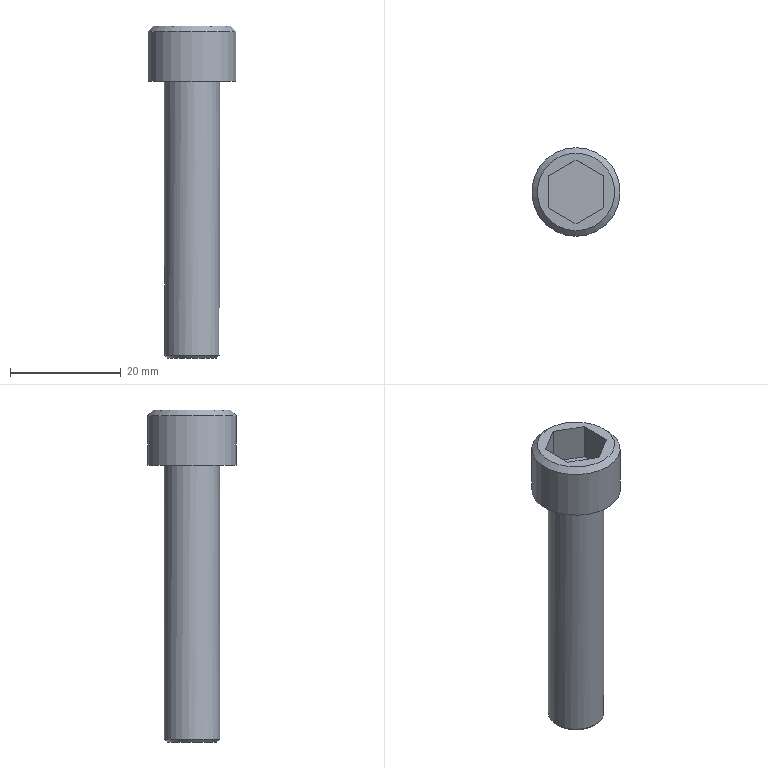Part | NX | features solid 2 | 1 solid | 14 faces | box 16 x 16 x 60 mm | volume 5332 mm3 | plane 10 | cylinder 2 | cone 2 | commonest cylinder face diameters 10 x1 16 x1
STEP:
#1=CARTESIAN_POINT('',(43.,472.,-31.));
#2=VERTEX_POINT('',#1);
#3=CARTESIAN_POINT('',(43.,480.,-31.));
#4=DIRECTION('',(0.,0.,1.));
#5=DIRECTION('',(0.,-1.,0.));
#6=AXIS2_PLACEMENT_3D('',#3,#4,#5);
#7=CIRCLE('',#6,8.);
#8=EDGE_CURVE('',#2,#2,#7,.F.);
#9=ORIENTED_EDGE('',*,*,#8,.T.);
#10=EDGE_LOOP('',(#9));
#11=FACE_BOUND('',#10,.T.);
#12=CARTESIAN_POINT('',(43.,472.,-40.));
#13=VERTEX_POINT('',#12);
#14=CARTESIAN_POINT('',(43.,480.,-40.));
#15=DIRECTION('',(0.,0.,1.));
#16=DIRECTION('',(0.,-1.,0.));
#17=AXIS2_PLACEMENT_3D('',#14,#15,#16);
#18=CIRCLE('',#17,8.);
#19=EDGE_CURVE('',#13,#13,#18,.T.);
#20=ORIENTED_EDGE('',*,*,#19,.T.);
#21=EDGE_LOOP('',(#20));
#22=FACE_BOUND('',#21,.T.);
#23=CARTESIAN_POINT('',(43.,480.,-40.));
#24=DIRECTION('',(0.,0.,1.));
#25=DIRECTION('',(0.,-1.,0.));
#26=AXIS2_PLACEMENT_3D('',#23,#24,#25);
#27=CYLINDRICAL_SURFACE('',#26,8.);
#28=ADVANCED_FACE('',(#11,#22),#27,.T.);
#29=CARTESIAN_POINT('',(48.,480.,-40.));
#30=VERTEX_POINT('',#29);
#31=CARTESIAN_POINT('',(43.,480.,-40.));
#32=DIRECTION('',(0.,0.,1.));
#33=DIRECTION('',(1.,0.,0.));
#34=AXIS2_PLACEMENT_3D('',#31,#32,#33);
#35=CIRCLE('',#34,5.);
#36=EDGE_CURVE('',#30,#30,#35,.F.);
#37=ORIENTED_EDGE('',*,*,#36,.F.);
#38=EDGE_LOOP('',(#37));
#39=FACE_BOUND('',#38,.T.);
#40=ORIENTED_EDGE('',*,*,#19,.F.);
#41=EDGE_LOOP('',(#40));
#42=FACE_BOUND('',#41,.T.);
#43=CARTESIAN_POINT('',(43.,480.,-40.));
#44=DIRECTION('',(0.,0.,1.));
#45=DIRECTION('',(0.,-1.,0.));
#46=AXIS2_PLACEMENT_3D('',#43,#44,#45);
#47=PLANE('',#46);
#48=ADVANCED_FACE('',(#39,#42),#47,.F.);
#49=CARTESIAN_POINT('',(43.,473.,-30.));
#50=VERTEX_POINT('',#49);
#51=CARTESIAN_POINT('',(43.,480.,-30.));
#52=DIRECTION('',(0.,0.,1.));
#53=DIRECTION('',(0.,-1.,0.));
#54=AXIS2_PLACEMENT_3D('',#51,#52,#53);
#55=CIRCLE('',#54,7.);
#56=EDGE_CURVE('',#50,#50,#55,.T.);
#57=ORIENTED_EDGE('',*,*,#56,.T.);
#58=EDGE_LOOP('',(#57));
#59=FACE_BOUND('',#58,.T.);
#60=CARTESIAN_POINT('',(48.,482.887,-30.));
#61=VERTEX_POINT('',#60);
#62=CARTESIAN_POINT('',(43.,485.774,-30.));
#63=VERTEX_POINT('',#62);
#64=CARTESIAN_POINT('',(48.,482.887,-30.));
#65=DIRECTION('',(-0.866,0.5,0.));
#66=VECTOR('',#65,1000.);
#67=LINE('',#64,#66);
#68=EDGE_CURVE('',#61,#63,#67,.T.);
#69=ORIENTED_EDGE('',*,*,#68,.F.);
#70=CARTESIAN_POINT('',(48.,477.113,-30.));
#71=VERTEX_POINT('',#70);
#72=CARTESIAN_POINT('',(48.,477.113,-30.));
#73=DIRECTION('',(0.,1.,0.));
#74=VECTOR('',#73,1000.);
#75=LINE('',#72,#74);
#76=EDGE_CURVE('',#71,#61,#75,.T.);
#77=ORIENTED_EDGE('',*,*,#76,.F.);
#78=CARTESIAN_POINT('',(43.,474.226,-30.));
#79=VERTEX_POINT('',#78);
#80=CARTESIAN_POINT('',(43.,474.226,-30.));
#81=DIRECTION('',(0.866,0.5,0.));
#82=VECTOR('',#81,1000.);
#83=LINE('',#80,#82);
#84=EDGE_CURVE('',#79,#71,#83,.T.);
#85=ORIENTED_EDGE('',*,*,#84,.F.);
#86=CARTESIAN_POINT('',(38.,477.113,-30.));
#87=VERTEX_POINT('',#86);
#88=CARTESIAN_POINT('',(38.,477.113,-30.));
#89=DIRECTION('',(0.866,-0.5,0.));
#90=VECTOR('',#89,1000.);
#91=LINE('',#88,#90);
#92=EDGE_CURVE('',#87,#79,#91,.T.);
#93=ORIENTED_EDGE('',*,*,#92,.F.);
#94=CARTESIAN_POINT('',(38.,482.887,-30.));
#95=VERTEX_POINT('',#94);
#96=CARTESIAN_POINT('',(38.,482.887,-30.));
#97=DIRECTION('',(0.,-1.,0.));
#98=VECTOR('',#97,1000.);
#99=LINE('',#96,#98);
#100=EDGE_CURVE('',#95,#87,#99,.T.);
#101=ORIENTED_EDGE('',*,*,#100,.F.);
#102=CARTESIAN_POINT('',(43.,485.774,-30.));
#103=DIRECTION('',(-0.866,-0.5,0.));
#104=VECTOR('',#103,1000.);
#105=LINE('',#102,#104);
#106=EDGE_CURVE('',#63,#95,#105,.T.);
#107=ORIENTED_EDGE('',*,*,#106,.F.);
#108=EDGE_LOOP('',(#69,#77,#85,#93,#101,#107));
#109=FACE_BOUND('',#108,.T.);
#110=CARTESIAN_POINT('',(43.,480.,-30.));
#111=DIRECTION('',(0.,0.,1.));
#112=DIRECTION('',(0.,-1.,0.));
#113=AXIS2_PLACEMENT_3D('',#110,#111,#112);
#114=PLANE('',#113);
#115=ADVANCED_FACE('',(#59,#109),#114,.T.);
#116=CARTESIAN_POINT('',(43.,484.5,-90.));
#117=VERTEX_POINT('',#116);
#118=CARTESIAN_POINT('',(43.,480.,-90.));
#119=DIRECTION('',(0.,0.,-1.));
#120=DIRECTION('',(0.,1.,0.));
#121=AXIS2_PLACEMENT_3D('',#118,#119,#120);
#122=CIRCLE('',#121,4.5);
#123=EDGE_CURVE('',#117,#117,#122,.T.);
#124=ORIENTED_EDGE('',*,*,#123,.T.);
#125=EDGE_LOOP('',(#124));
#126=FACE_BOUND('',#125,.T.);
#127=CARTESIAN_POINT('',(43.,480.,-90.));
#128=DIRECTION('',(0.,0.,-1.));
#129=DIRECTION('',(0.,1.,0.));
#130=AXIS2_PLACEMENT_3D('',#127,#128,#129);
#131=PLANE('',#130);
#132=ADVANCED_FACE('',(#126),#131,.T.);
#133=CARTESIAN_POINT('',(43.,485.,-89.5));
#134=VERTEX_POINT('',#133);
#135=CARTESIAN_POINT('',(43.,480.,-89.5));
#136=DIRECTION('',(0.,0.,-1.));
#137=DIRECTION('',(0.,1.,0.));
#138=AXIS2_PLACEMENT_3D('',#135,#136,#137);
#139=CIRCLE('',#138,5.);
#140=EDGE_CURVE('',#134,#134,#139,.F.);
#141=ORIENTED_EDGE('',*,*,#140,.T.);
#142=EDGE_LOOP('',(#141));
#143=FACE_BOUND('',#142,.T.);
#144=ORIENTED_EDGE('',*,*,#36,.T.);
#145=EDGE_LOOP('',(#144));
#146=FACE_BOUND('',#145,.T.);
#147=CARTESIAN_POINT('',(43.,480.,-55.));
#148=DIRECTION('',(0.,0.,-1.));
#149=DIRECTION('',(0.,1.,0.));
#150=AXIS2_PLACEMENT_3D('',#147,#148,#149);
#151=CYLINDRICAL_SURFACE('',#150,5.);
#152=ADVANCED_FACE('',(#143,#146),#151,.T.);
#153=ORIENTED_EDGE('',*,*,#68,.T.);
#154=CARTESIAN_POINT('',(43.,485.774,-36.667));
#155=VERTEX_POINT('',#154);
#156=CARTESIAN_POINT('',(43.,485.774,-36.667));
#157=DIRECTION('',(0.,0.,1.));
#158=VECTOR('',#157,1000.);
#159=LINE('',#156,#158);
#160=EDGE_CURVE('',#155,#63,#159,.T.);
#161=ORIENTED_EDGE('',*,*,#160,.F.);
#162=CARTESIAN_POINT('',(48.,482.887,-36.667));
#163=VERTEX_POINT('',#162);
#164=CARTESIAN_POINT('',(48.,482.887,-36.667));
#165=DIRECTION('',(-0.866,0.5,0.));
#166=VECTOR('',#165,1000.);
#167=LINE('',#164,#166);
#168=EDGE_CURVE('',#163,#155,#167,.T.);
#169=ORIENTED_EDGE('',*,*,#168,.F.);
#170=CARTESIAN_POINT('',(48.,482.887,-36.667));
#171=DIRECTION('',(0.,0.,1.));
#172=VECTOR('',#171,1000.);
#173=LINE('',#170,#172);
#174=EDGE_CURVE('',#163,#61,#173,.T.);
#175=ORIENTED_EDGE('',*,*,#174,.T.);
#176=EDGE_LOOP('',(#153,#161,#169,#175));
#177=FACE_BOUND('',#176,.T.);
#178=CARTESIAN_POINT('',(48.,482.887,-36.667));
#179=DIRECTION('',(0.5,0.866,0.));
#180=DIRECTION('',(-0.866,0.5,0.));
#181=AXIS2_PLACEMENT_3D('',#178,#179,#180);
#182=PLANE('',#181);
#183=ADVANCED_FACE('',(#177),#182,.F.);
#184=ORIENTED_EDGE('',*,*,#106,.T.);
#185=CARTESIAN_POINT('',(38.,482.887,-36.667));
#186=VERTEX_POINT('',#185);
#187=CARTESIAN_POINT('',(38.,482.887,-36.667));
#188=DIRECTION('',(0.,0.,1.));
#189=VECTOR('',#188,1000.);
#190=LINE('',#187,#189);
#191=EDGE_CURVE('',#186,#95,#190,.T.);
#192=ORIENTED_EDGE('',*,*,#191,.F.);
#193=CARTESIAN_POINT('',(43.,485.774,-36.667));
#194=DIRECTION('',(-0.866,-0.5,0.));
#195=VECTOR('',#194,1000.);
#196=LINE('',#193,#195);
#197=EDGE_CURVE('',#155,#186,#196,.T.);
#198=ORIENTED_EDGE('',*,*,#197,.F.);
#199=ORIENTED_EDGE('',*,*,#160,.T.);
#200=EDGE_LOOP('',(#184,#192,#198,#199));
#201=FACE_BOUND('',#200,.T.);
#202=CARTESIAN_POINT('',(43.,485.774,-36.667));
#203=DIRECTION('',(-0.5,0.866,0.));
#204=DIRECTION('',(-0.866,-0.5,0.));
#205=AXIS2_PLACEMENT_3D('',#202,#203,#204);
#206=PLANE('',#205);
#207=ADVANCED_FACE('',(#201),#206,.F.);
#208=ORIENTED_EDGE('',*,*,#100,.T.);
#209=CARTESIAN_POINT('',(38.,477.113,-36.667));
#210=VERTEX_POINT('',#209);
#211=CARTESIAN_POINT('',(38.,477.113,-36.667));
#212=DIRECTION('',(0.,0.,1.));
#213=VECTOR('',#212,1000.);
#214=LINE('',#211,#213);
#215=EDGE_CURVE('',#210,#87,#214,.T.);
#216=ORIENTED_EDGE('',*,*,#215,.F.);
#217=CARTESIAN_POINT('',(38.,482.887,-36.667));
#218=DIRECTION('',(0.,-1.,0.));
#219=VECTOR('',#218,1000.);
#220=LINE('',#217,#219);
#221=EDGE_CURVE('',#186,#210,#220,.T.);
#222=ORIENTED_EDGE('',*,*,#221,.F.);
#223=ORIENTED_EDGE('',*,*,#191,.T.);
#224=EDGE_LOOP('',(#208,#216,#222,#223));
#225=FACE_BOUND('',#224,.T.);
#226=CARTESIAN_POINT('',(38.,482.887,-36.667));
#227=DIRECTION('',(-1.,0.,0.));
#228=DIRECTION('',(0.,0.,-1.));
#229=AXIS2_PLACEMENT_3D('',#226,#227,#228);
#230=PLANE('',#229);
#231=ADVANCED_FACE('',(#225),#230,.F.);
#232=ORIENTED_EDGE('',*,*,#92,.T.);
#233=CARTESIAN_POINT('',(43.,474.226,-36.667));
#234=VERTEX_POINT('',#233);
#235=CARTESIAN_POINT('',(43.,474.226,-36.667));
#236=DIRECTION('',(0.,0.,1.));
#237=VECTOR('',#236,1000.);
#238=LINE('',#235,#237);
#239=EDGE_CURVE('',#234,#79,#238,.T.);
#240=ORIENTED_EDGE('',*,*,#239,.F.);
#241=CARTESIAN_POINT('',(38.,477.113,-36.667));
#242=DIRECTION('',(0.866,-0.5,0.));
#243=VECTOR('',#242,1000.);
#244=LINE('',#241,#243);
#245=EDGE_CURVE('',#210,#234,#244,.T.);
#246=ORIENTED_EDGE('',*,*,#245,.F.);
#247=ORIENTED_EDGE('',*,*,#215,.T.);
#248=EDGE_LOOP('',(#232,#240,#246,#247));
#249=FACE_BOUND('',#248,.T.);
#250=CARTESIAN_POINT('',(38.,477.113,-36.667));
#251=DIRECTION('',(-0.5,-0.866,0.));
#252=DIRECTION('',(0.866,-0.5,0.));
#253=AXIS2_PLACEMENT_3D('',#250,#251,#252);
#254=PLANE('',#253);
#255=ADVANCED_FACE('',(#249),#254,.F.);
#256=ORIENTED_EDGE('',*,*,#84,.T.);
#257=CARTESIAN_POINT('',(48.,477.113,-36.667));
#258=VERTEX_POINT('',#257);
#259=CARTESIAN_POINT('',(48.,477.113,-36.667));
#260=DIRECTION('',(0.,0.,1.));
#261=VECTOR('',#260,1000.);
#262=LINE('',#259,#261);
#263=EDGE_CURVE('',#258,#71,#262,.T.);
#264=ORIENTED_EDGE('',*,*,#263,.F.);
#265=CARTESIAN_POINT('',(43.,474.226,-36.667));
#266=DIRECTION('',(0.866,0.5,0.));
#267=VECTOR('',#266,1000.);
#268=LINE('',#265,#267);
#269=EDGE_CURVE('',#234,#258,#268,.T.);
#270=ORIENTED_EDGE('',*,*,#269,.F.);
#271=ORIENTED_EDGE('',*,*,#239,.T.);
#272=EDGE_LOOP('',(#256,#264,#270,#271));
#273=FACE_BOUND('',#272,.T.);
#274=CARTESIAN_POINT('',(43.,474.226,-36.667));
#275=DIRECTION('',(0.5,-0.866,0.));
#276=DIRECTION('',(0.866,0.5,0.));
#277=AXIS2_PLACEMENT_3D('',#274,#275,#276);
#278=PLANE('',#277);
#279=ADVANCED_FACE('',(#273),#278,.F.);
#280=ORIENTED_EDGE('',*,*,#76,.T.);
#281=ORIENTED_EDGE('',*,*,#174,.F.);
#282=CARTESIAN_POINT('',(48.,477.113,-36.667));
#283=DIRECTION('',(0.,1.,0.));
#284=VECTOR('',#283,1000.);
#285=LINE('',#282,#284);
#286=EDGE_CURVE('',#258,#163,#285,.T.);
#287=ORIENTED_EDGE('',*,*,#286,.F.);
#288=ORIENTED_EDGE('',*,*,#263,.T.);
#289=EDGE_LOOP('',(#280,#281,#287,#288));
#290=FACE_BOUND('',#289,.T.);
#291=CARTESIAN_POINT('',(48.,477.113,-36.667));
#292=DIRECTION('',(1.,0.,0.));
#293=DIRECTION('',(0.,1.,0.));
#294=AXIS2_PLACEMENT_3D('',#291,#292,#293);
#295=PLANE('',#294);
#296=ADVANCED_FACE('',(#290),#295,.F.);
#297=ORIENTED_EDGE('',*,*,#168,.T.);
#298=ORIENTED_EDGE('',*,*,#197,.T.);
#299=ORIENTED_EDGE('',*,*,#221,.T.);
#300=ORIENTED_EDGE('',*,*,#245,.T.);
#301=ORIENTED_EDGE('',*,*,#269,.T.);
#302=ORIENTED_EDGE('',*,*,#286,.T.);
#303=EDGE_LOOP('',(#297,#298,#299,#300,#301,#302));
#304=FACE_BOUND('',#303,.T.);
#305=CARTESIAN_POINT('',(43.,485.774,-36.667));
#306=DIRECTION('',(0.,0.,1.));
#307=DIRECTION('',(0.,-1.,0.));
#308=AXIS2_PLACEMENT_3D('',#305,#306,#307);
#309=PLANE('',#308);
#310=ADVANCED_FACE('',(#304),#309,.T.);
#311=ORIENTED_EDGE('',*,*,#8,.F.);
#312=EDGE_LOOP('',(#311));
#313=FACE_BOUND('',#312,.T.);
#314=ORIENTED_EDGE('',*,*,#56,.F.);
#315=EDGE_LOOP('',(#314));
#316=FACE_BOUND('',#315,.T.);
#317=CARTESIAN_POINT('',(43.,480.,-30.));
#318=DIRECTION('',(0.,0.,-1.));
#319=DIRECTION('',(0.,1.,0.));
#320=AXIS2_PLACEMENT_3D('',#317,#318,#319);
#321=CONICAL_SURFACE('',#320,7.,0.7854);
#322=ADVANCED_FACE('',(#313,#316),#321,.T.);
#323=ORIENTED_EDGE('',*,*,#140,.F.);
#324=EDGE_LOOP('',(#323));
#325=FACE_BOUND('',#324,.T.);
#326=ORIENTED_EDGE('',*,*,#123,.F.);
#327=EDGE_LOOP('',(#326));
#328=FACE_BOUND('',#327,.T.);
#329=CARTESIAN_POINT('',(43.,480.,-90.));
#330=DIRECTION('',(0.,0.,1.));
#331=DIRECTION('',(0.,-1.,0.));
#332=AXIS2_PLACEMENT_3D('',#329,#330,#331);
#333=CONICAL_SURFACE('',#332,4.5,0.7854);
#334=ADVANCED_FACE('',(#325,#328),#333,.T.);
#335=CLOSED_SHELL('',(#28,#48,#115,#132,#152,#183,#207,#231,#255,#279,#296,#310,#322,#334));
#336=MANIFOLD_SOLID_BREP('',#335);
#337=(LENGTH_UNIT()NAMED_UNIT(*)SI_UNIT(.MILLI.,.METRE.));
#338=UNCERTAINTY_MEASURE_WITH_UNIT(LENGTH_MEASURE(0.00001),#337,'','');
#339=(NAMED_UNIT(*)PLANE_ANGLE_UNIT()SI_UNIT($,.RADIAN.));
#340=(NAMED_UNIT(*)SI_UNIT($,.STERADIAN.)SOLID_ANGLE_UNIT());
#341=(GEOMETRIC_REPRESENTATION_CONTEXT(3)GLOBAL_UNCERTAINTY_ASSIGNED_CONTEXT((#338))GLOBAL_UNIT_ASSIGNED_CONTEXT((#337,#339,#340))REPRESENTATION_CONTEXT('',''));
#342=ADVANCED_BREP_SHAPE_REPRESENTATION('',(#336),#341);